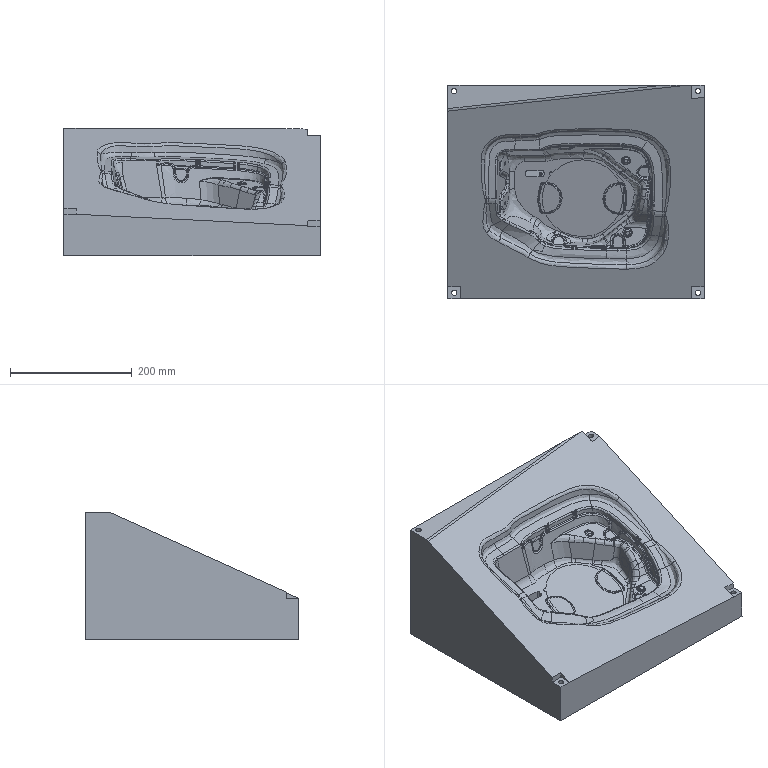NC program | NX | posted with a generic post | part box 420 x 350 x 208.3 mm
Lines 76212 to 77162 of 93858:
(CAVITY_MILL_COPY_COPY , TOOL : B10)
N152416 M6
N152418 G54
N152420 G17 G0 G90 X-24.596 Y68.606 S1900 M3
N152422 G43 Z220. H0
N152424 Z144.013
N152426 G94 G1 Z143.813 F3000.
N152428 X-24.626 Y69.131
N152430 G3 X-26.737 Y71.013 R2.
N152432 G1 X-27.419 Y70.974
N152434 G2 X-28.982 Y69.714 R8.488
N152436 G3 X-29.614 Y66.957 R2.
N152438 G1 X-29.446 Y66.689
N152440 Z144.013
N152442 G0 Z208.6
N152444 X-24.184 Y68.622
N152446 Z143.713
N152448 G1 Z143.513
N152450 X-24.214 Y69.156
N152452 G3 X-26.327 Y71.037 R2.
N152454 G1 X-27.167 Y70.988
N152456 G2 X-28.833 Y69.636 R8.726
N152458 G3 X-29.47 Y66.88 R2.
N152460 G1 X-29.3 Y66.608
N152462 Z143.713
N152464 G0 Z144.113
N152466 X-23.794 Y68.651
N152468 Z143.413
N152470 G1 Z143.213
N152472 X-23.818 Y69.15
N152474 G3 X-25.91 Y71.053 R2.
N152476 G1 X-26.569 Y71.022
N152478 X-26.917 Y71.002
N152480 G2 X-28.766 Y69.51 R8.706
N152482 G3 X-29.447 Y66.765 R2.
N152484 G1 X-29.282 Y66.491
N152486 Z143.413
N152488 G0 Z143.813
N152490 X-23.345 Y68.655
N152492 Z143.113
N152494 G1 Z142.913
N152496 X-23.365 Y69.155
N152498 G3 X-25.442 Y71.074 R2.
N152500 G1 X-26.179 Y71.045
N152502 X-26.699 Y71.014
N152504 G2 X-28.699 Y69.388 R8.526
N152506 G3 X-29.411 Y66.65 R2.
N152508 G1 X-29.25 Y66.377
N152510 Z143.113
N152512 G0 Z143.513
N152514 X-22.975 Y68.655
N152516 Z142.813
N152518 G1 Z142.613
N152520 X-23. Y69.154
N152522 G3 X-25.097 Y71.053 R2.
N152524 G1 X-26.52 Y70.982
N152526 G2 X-27.871 Y69.77 R8.475
N152528 G3 X-28.326 Y66.979 R2.
N152530 G1 X-28.141 Y66.722
N152532 Z142.813
N152534 G0 Z143.213
N152536 X-22.85 Y68.582
N152538 Z142.513
N152540 G1 Z142.313
N152542 X-22.875 Y69.084
N152544 G3 X-24.973 Y70.981 R2.
N152546 X-26.401 Y70.907 R693.689
N152548 G2 X-27.569 Y69.827 R8.285
N152550 G3 X-27.949 Y67.024 R2.
N152552 G1 X-27.76 Y66.775
N152554 Z142.513
N152556 G0 Z142.913
N152558 X-22.785 Y68.497
N152560 Z142.213
N152562 G1 Z142.013
N152564 X-22.809 Y68.998
N152566 G3 X-24.903 Y70.9 R2.
N152568 X-26.286 Y70.833 R1187.342
N152570 G2 X-27.347 Y69.835 R8.267
N152572 G3 X-27.683 Y67.027 R2.
N152574 G1 X-27.49 Y66.781
N152576 Z142.213
N152578 G0 Z142.613
N152580 X-22.687 Y68.421
N152582 Z141.913
N152584 G1 Z141.713
N152586 X-22.711 Y68.922
N152588 G3 X-24.804 Y70.824 R2.
N152590 X-26.172 Y70.758 R1216.244
N152592 G2 X-27.272 Y69.742 R8.44
N152594 G3 X-27.635 Y66.937 R2.
N152596 G1 X-27.442 Y66.687
N152598 Z141.913
N152600 G0 Z142.313
N152602 X-22.555 Y68.357
N152604 Z141.613
N152606 G1 Z141.413
N152608 X-22.581 Y68.862
N152610 G3 X-24.681 Y70.756 R2.
N152612 G1 X-26.066 Y70.684
N152614 G2 X-27.087 Y69.733 R8.336
N152616 G3 X-27.423 Y66.925 R2.
N152618 G1 X-27.23 Y66.678
N152620 Z141.613
N152622 G0 Z142.013
N152624 X-22.506 Y68.28
N152626 Z141.313
N152628 G1 Z141.113
N152630 X-22.531 Y68.779
N152632 G3 X-24.629 Y70.676 R2.
N152634 G1 X-25.967 Y70.609
N152636 G2 X-26.885 Y69.748 R8.451
N152638 G3 X-27.186 Y66.936 R2.
N152640 G1 X-26.987 Y66.69
N152642 Z141.313
N152644 G0 Z141.713
N152646 X-22.35 Y68.195
N152648 Z141.013
N152650 G1 Z140.813
N152652 X-22.373 Y68.696
N152654 G3 X-24.464 Y70.601 R2.
N152656 X-25.895 Y70.533 R1288.553
N152658 G2 X-26.753 Y69.72 R8.313
N152660 G3 X-27.03 Y66.905 R2.
N152662 G1 X-26.831 Y66.663
N152664 Z141.013
N152666 G0 Z141.413
N152668 X-22.395 Y68.125
N152670 Z140.713
N152672 G1 Z140.513
N152674 X-22.42 Y68.624
N152676 G3 X-24.518 Y70.522 R2.
N152678 G1 X-25.81 Y70.457
N152680 G2 X-26.608 Y69.701 R8.313
N152682 G3 X-26.871 Y66.885 R2.
N152684 G1 X-26.671 Y66.643
N152686 Z140.713
N152688 G0 Z141.113
N152690 X-22.336 Y68.049
N152692 Z140.413
N152694 G1 Z140.213
N152696 X-22.361 Y68.549
N152698 G3 X-24.459 Y70.445 R2.
N152700 G1 X-25.73 Y70.381
N152702 G2 X-26.499 Y69.657 R8.357
N152704 G3 X-26.763 Y66.841 R2.
N152706 G1 X-26.563 Y66.599
N152708 Z140.413
N152710 G0 Z140.813
N152712 X-22.29 Y67.968
N152714 Z140.113
N152716 G1 Z139.913
N152718 X-22.317 Y68.476
N152720 G3 X-24.418 Y70.369 R2.
N152722 G1 X-25.659 Y70.304
N152724 G2 X-26.372 Y69.632 R8.336
N152726 G3 X-26.621 Y66.815 R2.
N152728 G1 X-26.42 Y66.574
N152730 Z140.113
N152732 G0 Z140.513
N152734 X-22.224 Y67.897
N152736 Z139.813
N152738 G1 Z139.613
N152740 X-22.25 Y68.397
N152742 G3 X-24.35 Y70.291 R2.
N152744 G1 X-25.617 Y70.226
N152746 G2 X-26.283 Y69.593 R8.232
N152748 G3 X-26.515 Y66.774 R2.
N152750 G1 X-26.313 Y66.536
N152752 Z139.813
N152754 G0 Z140.213
N152756 X-22.246 Y67.818
N152758 Z139.513
N152760 G1 Z139.313
N152762 X-22.272 Y68.317
N152764 G3 X-24.373 Y70.21 R2.
N152766 G1 X-25.562 Y70.148
N152768 G2 X-26.205 Y69.543 R8.285
N152770 G3 X-26.441 Y66.725 R2.
N152772 G1 X-26.239 Y66.486
N152774 Z139.513
N152776 G0 Z139.913
N152778 X-22.277 Y67.737
N152780 Z139.213
N152782 G1 Z139.013
N152784 X-22.303 Y68.237
N152786 G3 X-24.406 Y70.129 R2.
N152788 G1 X-25.518 Y70.07
N152790 G2 X-26.098 Y69.523 R8.284
N152792 G3 X-26.318 Y66.704 R2.
N152794 G1 X-26.114 Y66.466
N152796 Z139.213
N152798 G0 Z139.613
N152800 X-22.359 Y67.654
N152802 Z138.913
N152804 G1 Z138.713
N152806 X-22.386 Y68.154
N152808 G3 X-24.489 Y70.044 R2.
N152810 G1 X-25.48 Y69.992
N152812 G2 X-26. Y69.5 R8.253
N152814 G3 X-26.202 Y66.679 R2.
N152816 G1 X-25.998 Y66.443
N152818 Z138.913
N152820 G0 Z139.313
N152822 X-22.463 Y67.559
N152824 Z138.614
N152826 G1 Z138.414
N152828 X-22.488 Y68.059
N152830 G3 X-24.585 Y69.957 R2.
N152832 G1 X-25.443 Y69.914
N152834 G2 X-25.905 Y69.478 R8.28
N152836 G3 X-26.096 Y66.656 R2.
N152838 G1 X-25.89 Y66.421
N152840 Z138.614
N152842 G0 Z139.013
N152844 X-21.214 Y67.536
N152846 Z138.314
N152848 G1 Z138.114
N152850 X-21.237 Y68.037
N152852 G3 X-23.329 Y69.941 R2.
N152854 X-25.423 Y69.84 R942.677
N152856 G2 X-26.653 Y68.814 R8.248
N152858 G3 X-27.182 Y66.035 R2.
N152860 G1 X-27.006 Y65.777
N152862 Z138.314
N152864 G0 Z138.714
N152866 X-21.185 Y67.466
N152868 Z138.014
N152870 G1 Z137.814
N152872 X-21.208 Y67.967
N152874 G3 X-23.298 Y69.873 R2.
N152876 X-25.387 Y69.774 R1000.498
N152878 G2 X-26.617 Y68.754 R8.221
N152880 G3 X-27.152 Y65.976 R2.
N152882 G1 X-26.977 Y65.718
N152884 Z138.014
N152886 G0 Z138.414
N152888 X-21.162 Y67.4
N152890 Z137.714
N152892 G1 Z137.514
N152894 X-21.185 Y67.901
N152896 G3 X-23.272 Y69.81 R2.
N152898 X-25.364 Y69.715 R1143.171
N152900 G2 X-26.596 Y68.694 R8.192
N152902 G3 X-27.133 Y65.917 R2.
N152904 G1 X-26.959 Y65.659
N152906 Z137.714
N152908 G0 Z138.114
N152910 X-21.658 Y67.322
N152912 Z137.414
N152914 G1 Z137.214
N152916 X-21.679 Y67.823
N152918 G3 X-23.762 Y69.736 R2.
N152920 G1 X-25.345 Y69.656
N152922 G2 X-26.217 Y68.892 R8.146
N152924 G3 X-26.604 Y66.09 R2.
N152926 G1 X-26.416 Y65.843
N152928 Z137.414
N152930 G0 Z137.814
N152932 X-21.11 Y67.287
N152934 Z137.114
N152936 G1 Z136.914
N152938 X-21.133 Y67.797
N152940 G3 X-23.221 Y69.704 R2.
N152942 X-25.326 Y69.596 R177.448
N152944 G2 X-26.544 Y68.585 R8.113
N152946 G3 X-27.079 Y65.807 R2.
N152948 G1 X-26.905 Y65.551
N152950 Z137.114
N152952 G0 Z137.514
N152954 X-21.097 Y67.234
N152956 Z136.814
N152958 G1 Z136.614
N152960 X-21.121 Y67.745
N152962 G3 X-23.213 Y69.648 R2.
N152964 X-25.307 Y69.537 R177.82
N152966 G2 X-26.521 Y68.531 R8.117
N152968 G3 X-27.057 Y65.754 R2.
N152970 G1 X-26.883 Y65.497
N152972 Z136.814
N152974 G0 Z137.214
N152976 X-21.105 Y67.182
N152978 Z136.514
N152980 G1 Z136.314
N152982 X-21.134 Y67.703
N152984 G3 X-23.24 Y69.59 R2.
N152986 G1 X-25.287 Y69.478
N152988 G2 X-26.497 Y68.479 R8.142
N152990 G3 X-27.035 Y65.703 R2.
N152992 G1 X-26.862 Y65.446
N152994 Z136.514
N152996 G0 Z136.914
N152998 X-21.072 Y67.128
N153000 Z136.214
N153002 G1 Z136.014
N153004 X-21.1 Y67.649
N153006 G3 X-23.207 Y69.537 R2.
N153008 G1 X-25.263 Y69.424
N153010 G2 X-26.306 Y68.535 R7.935
N153012 G3 X-26.773 Y65.745 R2.
N153014 G1 X-26.595 Y65.496
N153016 Z136.214
N153018 G0 Z136.614
N153020 X-21.053 Y67.073
N153022 Z135.914
N153024 G1 Z135.714
N153026 X-21.081 Y67.594
N153028 G3 X-23.186 Y69.483 R2.
N153030 G1 X-25.236 Y69.373
N153032 G2 X-26.275 Y68.492 R8.03
N153034 G3 X-26.745 Y65.703 R2.
N153036 G1 X-26.566 Y65.451
N153038 Z135.914
N153040 G0 Z136.314
N153042 X-21.023 Y67.019
N153044 Z135.614
N153046 G1 Z135.414
N153048 X-21.05 Y67.539
N153050 G3 X-23.154 Y69.43 R2.
N153052 G1 X-25.209 Y69.321
N153054 G2 X-26.186 Y68.483 R8.026
N153056 G3 X-26.628 Y65.689 R2.
N153058 G1 X-26.447 Y65.44
N153060 Z135.614
N153062 G0 Z136.014
N153064 X-20.996 Y66.965
N153066 Z135.314
N153068 G1 Z135.114
N153070 X-21.023 Y67.484
N153072 G3 X-23.124 Y69.377 R2.
N153074 G1 X-25.182 Y69.27
N153076 G2 X-26.172 Y68.423 R8.034
N153078 G3 X-26.619 Y65.63 R2.
N153080 G1 X-26.438 Y65.38
N153082 Z135.314
N153084 G0 Z135.714
N153086 X-20.969 Y66.911
N153088 Z135.014
N153090 G1 Z134.814
N153092 X-20.996 Y67.429
N153094 G3 X-23.096 Y69.324 R2.
N153096 G1 X-25.155 Y69.219
N153098 G2 X-26.164 Y68.358 R8.052
N153100 G3 X-26.62 Y65.567 R2.
N153102 G1 X-26.44 Y65.316
N153104 Z135.014
N153106 G0 Z135.414
N153108 X-20.944 Y66.856
N153110 Z134.714
N153112 G1 Z134.514
N153114 X-20.97 Y67.374
N153116 G3 X-23.069 Y69.271 R2.
N153118 G1 X-25.128 Y69.167
N153120 G2 X-26.167 Y68.287 R8.084
N153122 G3 X-26.637 Y65.498 R2.
N153124 G1 X-26.458 Y65.246
N153126 Z134.714
N153128 G0 Z135.114
N153130 X-20.919 Y66.802
N153132 Z134.414
N153134 G1 Z134.214
N153136 X-20.944 Y67.319
N153138 G3 X-23.041 Y69.218 R2.
N153140 G1 X-25.101 Y69.116
N153142 G2 X-26.17 Y68.216 R8.106
N153144 G3 X-26.653 Y65.429 R2.
N153146 G1 X-26.475 Y65.176
N153148 Z134.414
N153150 G0 Z134.814
N153152 X-20.87 Y66.741
N153154 Z134.114
N153156 G1 Z133.914
N153158 X-20.888 Y67.24
N153160 G3 X-22.96 Y69.166 R2.
N153162 G1 X-23.054 Y69.163
N153164 X-25.075 Y69.064
N153166 G2 X-26.159 Y68.154 R8.108
N153168 G3 X-26.65 Y65.368 R2.
N153170 G1 X-26.472 Y65.114
N153172 Z134.114
N153174 G0 Z134.514
N153176 X-20.828 Y66.69
N153178 Z133.814
N153180 G1 Z133.614
N153182 X-20.846 Y67.189
N153184 G3 X-22.918 Y69.115 R2.
N153186 G1 X-23.054 Y69.11
N153188 X-25.049 Y69.013
N153190 G2 X-26.12 Y68.111 R8.099
N153192 G3 X-26.605 Y65.325 R2.
N153194 G1 X-26.427 Y65.071
N153196 Z133.814
N153198 G0 Z134.214
N153200 X-20.796 Y66.638
N153202 Z133.515
N153204 G1 Z133.315
N153206 X-20.814 Y67.138
N153208 G3 X-22.885 Y69.063 R2.
N153210 G1 X-23.054 Y69.057
N153212 X-25.023 Y68.961
N153214 G2 X-26.095 Y68.06 R8.111
N153216 G3 X-26.581 Y65.273 R2.
N153218 G1 X-26.403 Y65.02
N153220 Z133.515
N153222 G0 Z133.914
N153224 X-20.772 Y66.586
N153226 Z133.215
N153228 G1 Z133.015
N153230 X-20.791 Y67.086
N153232 G3 X-22.862 Y69.011 R2.
N153234 G1 X-23.054 Y69.004
N153236 X-24.997 Y68.91
N153238 G2 X-26.073 Y68.007 R8.129
N153240 G3 X-26.561 Y65.221 R2.
N153242 G1 X-26.383 Y64.967
N153244 Z133.215
N153246 G0 Z133.615
N153248 X-20.746 Y66.534
N153250 Z132.915
N153252 G1 Z132.715
N153254 X-20.764 Y67.034
N153256 G3 X-22.836 Y68.959 R2.
N153258 G1 X-23.054 Y68.952
N153260 X-24.971 Y68.859
N153262 G2 X-26.031 Y67.966 R8.119
N153264 G3 X-26.512 Y65.179 R2.
N153266 G1 X-26.333 Y64.926
N153268 Z132.915
N153270 G0 Z133.315
N153272 X-20.722 Y66.482
N153274 Z132.615
N153276 G1 Z132.415
N153278 X-20.74 Y66.982
N153280 G3 X-22.812 Y68.907 R2.
N153282 G1 X-23.054 Y68.899
N153284 X-24.945 Y68.807
N153286 G2 X-25.995 Y67.922 R8.129
N153288 G3 X-26.474 Y65.134 R2.
N153290 G1 X-26.295 Y64.881
N153292 Z132.615
N153294 G0 Z133.015
N153296 X-20.697 Y66.43
N153298 Z132.315
N153300 G1 Z132.115
N153302 X-20.715 Y66.93
N153304 G3 X-22.787 Y68.856 R2.
N153306 G1 X-23.054 Y68.846
N153308 X-24.919 Y68.756
N153310 G2 X-25.962 Y67.876 R8.13
N153312 G3 X-26.438 Y65.088 R2.
N153314 G1 X-26.258 Y64.834
N153316 Z132.315
N153318 G0 Z132.715
N153320 X-20.672 Y66.378
N153322 Z132.015
N153324 G1 Z131.815
N153326 X-20.691 Y66.878
N153328 G3 X-22.762 Y68.804 R2.
N153330 G1 X-23.054 Y68.793
N153332 X-24.893 Y68.704
N153334 G2 X-25.927 Y67.831 R8.138
N153336 G3 X-26.399 Y65.042 R2.
N153338 G1 X-26.219 Y64.789
N153340 Z132.015
N153342 G0 Z132.415
N153344 X-20.724 Y66.323
N153346 Z131.715
N153348 G1 Z131.515
N153350 X-20.742 Y66.823
N153352 G3 X-22.814 Y68.749 R2.
N153354 G1 X-23.054 Y68.74
N153356 X-24.867 Y68.653
N153358 G2 X-25.893 Y67.786 R8.143
N153360 G3 X-26.362 Y64.996 R2.
N153362 G1 X-26.182 Y64.744
N153364 Z131.715
N153366 G0 Z132.115
N153368 X-20.771 Y66.269
N153370 Z131.415
N153372 G1 Z131.215
N153374 X-20.789 Y66.768
N153376 G3 X-22.861 Y68.694 R2.
N153378 G1 X-23.054 Y68.687
N153380 X-24.84 Y68.601
N153382 G2 X-25.863 Y67.738 R8.162
N153384 G3 X-26.332 Y64.949 R2.
N153386 G1 X-26.152 Y64.695
N153388 Z131.415
N153390 G0 Z131.815
N153392 X-20.796 Y66.215
N153394 Z131.115
N153396 G1 Z130.915
N153398 X-20.815 Y66.715
N153400 G3 X-22.886 Y68.64 R2.
N153402 G1 X-23.054 Y68.634
N153404 X-24.814 Y68.55
N153406 G2 X-25.827 Y67.694 R8.173
N153408 G3 X-26.292 Y64.904 R2.
N153410 G1 X-26.112 Y64.651
N153412 Z131.115
N153414 G0 Z131.515
N153416 X-20.824 Y66.161
N153418 Z130.815
N153420 G1 Z130.615
N153422 X-20.842 Y66.661
N153424 G3 X-22.914 Y68.587 R2.
N153426 G1 X-23.054 Y68.581
N153428 X-24.788 Y68.499
N153430 G2 X-25.876 Y67.591 R8.183
N153432 G3 X-26.372 Y64.806 R2.
N153434 G1 X-26.194 Y64.551
N153436 Z130.815
N153438 G0 Z131.215
N153440 X-20.828 Y66.108
N153442 Z130.515
N153444 G1 Z130.315
N153446 X-20.846 Y66.608
N153448 G3 X-22.917 Y68.534 R2.
N153450 G1 X-23.054 Y68.529
N153452 X-24.762 Y68.447
N153454 G2 X-25.754 Y67.608 R8.2
N153456 G3 X-26.211 Y64.817 R2.
N153458 G1 X-26.029 Y64.564
N153460 Z130.515
N153462 G0 Z130.915
N153464 X-20.838 Y66.055
N153466 Z130.215
N153468 G1 Z130.015
N153470 X-20.857 Y66.554
N153472 G3 X-22.928 Y68.48 R2.
N153474 G1 X-23.054 Y68.476
N153476 X-24.736 Y68.396
N153478 G2 X-25.713 Y67.568 R8.212
N153480 G3 X-26.164 Y64.776 R2.
N153482 G1 X-25.982 Y64.523
N153484 Z130.215
N153486 G0 Z130.615
N153488 X-20.847 Y66.002
N153490 Z129.915
N153492 G1 Z129.715
N153494 X-20.865 Y66.501
N153496 G3 X-22.937 Y68.427 R2.
N153498 G1 X-23.054 Y68.423
N153500 X-24.71 Y68.344
N153502 G2 X-25.656 Y67.537 R8.164
N153504 G3 X-26.095 Y64.743 R2.
N153506 G1 X-25.912 Y64.492
N153508 Z129.915
N153510 G0 Z130.315
N153512 X-20.855 Y65.948
N153514 Z129.615
N153516 G1 Z129.415
N153518 X-20.873 Y66.448
N153520 G3 X-22.945 Y68.374 R2.
N153522 G1 X-23.054 Y68.37
N153524 X-24.684 Y68.293
N153526 G2 X-25.63 Y67.488 R8.232
N153528 G3 X-26.07 Y64.694 R2.
N153530 G1 X-25.887 Y64.442
N153532 Z129.615
N153534 G0 Z130.015
N153536 X-20.861 Y65.895
N153538 Z129.315
N153540 G1 Z129.115
N153542 X-20.879 Y66.395
N153544 G3 X-22.951 Y68.321 R2.
N153546 G1 X-23.054 Y68.317
N153548 X-24.658 Y68.241
N153550 G2 X-25.589 Y67.448 R8.242
N153552 G3 X-26.023 Y64.653 R2.
N153554 G1 X-25.839 Y64.401
N153556 Z129.315
N153558 G0 Z129.715
N153560 X-20.867 Y65.842
N153562 Z129.015
N153564 G1 Z128.815
N153566 X-20.885 Y66.342
N153568 G3 X-22.957 Y68.268 R2.
N153570 G1 X-23.054 Y68.264
N153572 X-24.632 Y68.19
N153574 G2 X-25.555 Y67.404 R8.253
N153576 G3 X-25.988 Y64.609 R2.
N153578 G1 X-25.803 Y64.357
N153580 Z129.015
N153582 G0 Z129.415
N153584 X-21.65 Y65.755
N153586 Z128.715
N153588 G1 Z128.515
N153590 X-21.669 Y66.254
N153592 G3 X-23.742 Y68.179 R2.
N153594 G1 X-23.835 Y68.175
N153596 X-24.606 Y68.138
N153598 G2 X-25.07 Y67.711 R8.17
N153600 G3 X-25.297 Y64.891 R2.
N153602 G1 X-25.095 Y64.655
N153604 Z128.715
N153606 G0 Z129.115
N153608 X-21.625 Y65.703
N153610 Z128.416
N153612 G1 Z128.216
N153614 X-21.644 Y66.202
N153616 G3 X-23.717 Y68.127 R2.
N153618 G1 X-23.835 Y68.123
N153620 X-24.58 Y68.087
N153622 G2 X-25.045 Y67.659 R8.17
N153624 G3 X-25.271 Y64.84 R2.
N153626 G1 X-25.07 Y64.603
N153628 Z128.416
N153630 G0 Z128.815
N153632 X-21.6 Y65.651
N153634 Z128.116
N153636 G1 Z127.916
N153638 X-21.619 Y66.151
N153640 G3 X-23.692 Y68.075 R2.
N153642 G1 X-23.835 Y68.07
N153644 X-24.554 Y68.035
N153646 G2 X-25.018 Y67.608 R8.168
N153648 G3 X-25.244 Y64.789 R2.
N153650 G1 X-25.043 Y64.552
N153652 Z128.116
N153654 G0 Z128.516
N153656 X-21.575 Y65.599
N153658 Z127.816
N153660 G1 Z127.616
N153662 X-21.594 Y66.099
N153664 G3 X-23.667 Y68.023 R2.
N153666 G1 X-23.835 Y68.017
N153668 X-24.528 Y67.984
N153670 G2 X-24.992 Y67.557 R8.173
N153672 G3 X-25.219 Y64.737 R2.
N153674 G1 X-25.018 Y64.5
N153676 Z127.816
N153678 G0 Z128.216
N153680 X-21.55 Y65.547
N153682 Z127.516
N153684 G1 Z127.316
N153686 X-21.569 Y66.047
N153688 G3 X-23.641 Y67.971 R2.
N153690 G1 X-23.835 Y67.964
N153692 X-24.502 Y67.932
N153694 G2 X-24.964 Y67.506 R8.149
N153696 G3 X-25.187 Y64.687 R2.
N153698 G1 X-24.986 Y64.451
N153700 Z127.516
N153702 G0 Z127.916
N153704 X-21.513 Y65.496
N153706 Z127.216
N153708 G1 Z127.016
N153710 X-21.531 Y65.995
N153712 G3 X-23.604 Y67.92 R2.
N153714 G1 X-23.835 Y67.911
N153716 X-24.476 Y67.881
N153718 G2 X-24.95 Y67.443 R8.125
N153720 G3 X-25.177 Y64.624 R2.
N153722 G1 X-24.976 Y64.388
N153724 Z127.216
N153726 G0 Z127.616
N153728 X-21.5 Y65.443
N153730 Z126.916
N153732 G1 Z126.716
N153734 X-21.519 Y65.943
N153736 G3 X-23.592 Y67.868 R2.
N153738 G1 X-23.835 Y67.858
N153740 X-24.448 Y67.829
N153742 G2 X-24.932 Y67.38 R7.975
N153744 G3 X-25.158 Y64.561 R2.
N153746 G1 X-24.959 Y64.327
N153748 Z126.916
N153750 G0 Z127.316
N153752 X-21.449 Y65.392
N153754 Z126.616
N153756 G1 Z126.416
N153758 X-21.467 Y65.892
N153760 G3 X-23.54 Y67.817 R2.
N153762 G1 X-23.835 Y67.806
N153764 X-24.421 Y67.778
N153766 G2 X-24.937 Y67.3 R7.939
N153768 G3 X-25.173 Y64.482 R2.
N153770 G1 X-24.975 Y64.248
N153772 Z126.616
N153774 G0 Z127.016
N153776 X-21.328 Y65.344
N153778 Z126.316
N153780 G1 Z126.116
N153782 X-21.346 Y65.844
N153784 G3 X-23.419 Y67.768 R2.
N153786 G1 X-23.835 Y67.753
N153788 X-24.373 Y67.727
N153790 G2 X-24.999 Y67.163 R8.033
N153792 G3 X-25.293 Y64.35 R2.
N153794 G1 X-25.099 Y64.111
N153796 Z126.316
N153798 G0 Z126.716
N153800 X-21.468 Y65.291
N153802 Z126.016
N153804 G1 Z125.816
N153806 X-21.492 Y65.804
N153808 G3 X-23.581 Y67.711 R2.
N153810 G1 X-24.326 Y67.677
N153812 G2 X-24.803 Y67.237 R8.039
N153814 G3 X-25.03 Y64.417 R2.
N153816 G1 X-24.83 Y64.182
N153818 Z126.016
N153820 G0 Z126.416
N153822 X-21.414 Y65.235
N153824 Z125.716
N153826 G1 Z125.516
N153828 X-21.433 Y65.735
N153830 G3 X-23.505 Y67.659 R2.
N153832 G1 X-23.835 Y67.647
N153834 X-24.278 Y67.626
N153836 G2 X-24.799 Y67.147 R7.995
N153838 G3 X-25.043 Y64.329 R2.
N153840 G1 X-24.845 Y64.094
N153842 Z125.716
N153844 G0 Z126.116
N153846 X-21.32 Y65.186
N153848 Z125.416
N153850 G1 Z125.216
N153852 X-21.338 Y65.686
N153854 G3 X-23.411 Y67.61 R2.
N153856 G1 X-23.835 Y67.594
N153858 X-24.209 Y67.577
N153860 G2 X-24.78 Y67.058 R8.04
N153862 G3 X-25.05 Y64.243 R2.
N153864 G1 X-24.854 Y64.005
N153866 Z125.416
N153868 G0 Z125.816
N153870 X-21.216 Y65.135
N153872 Z125.116
N153874 G1 Z124.916
N153876 X-21.235 Y65.635
N153878 G3 X-23.308 Y67.559 R2.
N153880 G1 X-24.101 Y67.529
N153882 G2 X-24.725 Y66.979 R8.316
N153884 G3 X-25.044 Y64.168 R2.
N153886 G1 X-24.848 Y63.923
N153888 Z125.116
N153890 G0 Z125.516
N153892 X-21.067 Y65.098
N153894 Z124.816
N153896 G1 Z124.616
N153898 X-21.088 Y65.605
N153900 G3 X-23.173 Y67.517 R2.
N153902 G1 X-23.996 Y67.481
N153904 G2 X-24.677 Y66.894 R8.526
N153906 G3 X-25.037 Y64.089 R2.
N153908 G1 X-24.843 Y63.838
N153910 Z124.816
N153912 G0 Z125.216
N153914 X-20.941 Y65.05
N153916 Z124.516
N153918 G1 Z124.316
N153920 X-20.963 Y65.558
N153922 G3 X-23.048 Y67.469 R2.
N153924 G1 X-23.892 Y67.433
N153926 G2 X-24.641 Y66.798 R8.595
N153928 G3 X-25.035 Y63.997 R2.
N153930 G1 X-24.843 Y63.743
N153932 Z124.516
N153934 G0 Z124.916
N153936 X-20.801 Y65.002
N153938 Z124.216
N153940 G1 Z124.016
N153942 X-20.823 Y65.51
N153944 G3 X-22.907 Y67.423 R2.
N153946 G1 X-23.775 Y67.385
N153948 G2 X-24.63 Y66.675 R8.668
N153950 G3 X-25.072 Y63.882 R2.
N153952 G1 X-24.884 Y63.623
N153954 Z124.216
N153956 G0 Z124.616
N153958 X-20.645 Y64.955
N153960 Z123.916
N153962 G1 Z123.716
N153964 X-20.667 Y65.464
N153966 G3 X-22.751 Y67.377 R2.
N153968 G1 X-23.619 Y67.339
N153970 G2 X-24.633 Y66.532 R8.953
N153972 G3 X-25.154 Y63.752 R2.
N153974 G1 X-24.971 Y63.485
N153976 Z123.916
N153978 G0 Z124.316
N153980 X-20.473 Y64.908
N153982 Z123.616
N153984 G1 Z123.416
N153986 X-20.495 Y65.418
N153988 G3 X-22.578 Y67.331 R2.
N153990 G1 X-23.463 Y67.293
N153992 G2 X-24.611 Y66.399 R8.841
N153994 G3 X-25.189 Y63.63 R2.
N153996 G1 X-25.013 Y63.36
N153998 Z123.616
N154000 G0 Z124.016
N154002 X-20.302 Y64.861
N154004 Z123.317
N154006 G1 Z123.117
N154008 X-20.324 Y65.372
N154010 G3 X-22.406 Y67.286 R2.
N154012 G1 X-23.265 Y67.249
N154014 G2 X-24.57 Y66.276 R9.205
N154016 G3 X-25.223 Y63.524 R2.
N154018 G1 X-25.051 Y63.244
N154020 Z123.317
N154022 G0 Z123.716
N154024 X-20.113 Y64.816
N154026 Z123.017
N154028 G1 Z122.817
N154030 X-20.131 Y65.315
N154032 G3 X-22.203 Y67.241 R2.
N154034 G1 X-23.057 Y67.206
N154036 G2 X-24.616 Y66.1 R9.526
N154038 G3 X-25.369 Y63.374 R2.
N154040 G1 X-25.205 Y63.085
N154042 Z123.017
N154044 G0 Z123.417
N154046 X-19.908 Y64.77
N154048 Z122.717
N154050 G1 Z122.517
N154052 X-19.926 Y65.27
N154054 G3 X-21.998 Y67.195 R2.
N154056 G1 X-22.272 Y67.185
N154058 X-22.792 Y67.164
N154060 G2 X-24.99 Y65.779 R10.597
N154062 G3 X-25.949 Y63.119 R2.
N154064 G1 X-25.802 Y62.805
N154066 Z122.717
N154068 G0 Z123.117
N154070 X-19.683 Y64.725
N154072 Z122.417
N154074 G1 Z122.217
N154076 X-19.701 Y65.225
N154078 G3 X-21.774 Y67.15 R2.
N154080 G1 X-22.518 Y67.122
N154082 G2 X-24.976 Y65.657 R12.08
N154084 G3 X-25.989 Y63.016 R2.
N154086 G1 X-25.847 Y62.697
N154088 Z122.417
N154090 G0 Z122.817
N154092 X-19.428 Y64.682
N154094 Z122.117
N154096 G1 Z121.917
N154098 X-19.447 Y65.182
N154100 G3 X-21.519 Y67.107 R2.
N154102 G1 X-22.245 Y67.08
N154104 G2 X-24.842 Y65.582 R11.939
N154106 G3 X-25.912 Y62.963 R2.
N154108 G1 X-25.773 Y62.631
N154110 Z122.117
N154112 G0 Z123.217
N154114 X77.643 Y53.74
N154116 Z121.217
N154118 G1 Z121.017
N154120 G3 X80.036 Y54.931 R2.
N154122 G2 X80.346 Y55.264 R0.627
N154124 X82.481 Y55.241 R1.437
N154126 G3 X85.123 Y54.92 R2.
N154128 G1 Z121.217
N154130 G0 Z121.617
N154132 X99.419 Y59.382
N154134 Z121.217
N154136 G1 Z121.017
N154138 X99.625 Y59.92
N154140 G3 X98.474 Y62.504 R2.
N154142 G1 X98.44 Y62.517
N154144 X58.723 Y56.193
N154146 G2 X55.461 Y56.234 R21.912
N154148 G3 X53.294 Y54.416 R2.
N154150 G1 X53.258 Y53.999
N154152 Z121.217
N154154 G0 Z121.617
N154156 X76.778 Y50.866
N154158 Z120.917
N154160 G1 Z120.717
N154162 G3 X77.996 Y53.408 R2.
N154164 G2 X77.905 Y53.91 R1.641
N154166 X78.508 Y55.812 R2.792
N154168 X84.554 Y55.829 R3.867
N154170 X84.581 Y53.531 R1.814
N154172 G3 X84.901 Y50.715 R2.
N154174 G1 Z120.917
N154176 G0 Z121.317
N154178 X100.805 Y58.63
N154180 Z120.917
N154182 G1 Z120.717
N154184 X101.042 Y59.177
N154186 G3 X100.002 Y61.807 R2.
N154188 G1 X99.953 Y61.828
N154190 X59.518 Y55.391
N154192 G2 X56.482 Y55.433 R18.77
N154194 G3 X54.301 Y53.631 R2.
N154196 G1 X54.263 Y53.227
N154198 Z120.917
N154200 G0 Z121.317
N154202 X76.151 Y49.646
N154204 Z120.617
N154206 G1 Z120.417
N154208 X76.217 Y49.68
N154210 G3 X77.046 Y52.384 R2.
N154212 G2 X76.766 Y53.489 R2.41
N154214 X79.402 Y57.627 R4.494
N154216 G1 X60.265 Y54.58
N154218 G2 X57.293 Y54.641 R16.305
N154220 G3 X55.082 Y52.877 R2.
N154222 G1 X55.038 Y52.486
N154224 Z120.617
N154226 G0 Z121.017
N154228 X75.651 Y48.665
N154230 Z120.317
N154232 G1 Z120.117
N154234 X75.741 Y48.719
N154236 G3 X76.431 Y51.461 R2.
N154238 G2 X76.165 Y52.059 R2.763
N154240 X76.848 Y56.291 R4.79
N154242 G1 X60.995 Y53.767
N154244 G2 X58.103 Y53.846 R13.352
N154246 G3 X55.85 Y52.135 R2.
N154248 G1 X55.799 Y51.759
N154250 Z120.317
N154252 G0 Z120.717
N154254 X77.992 Y46.7
N154256 Z120.017
N154258 G1 Z119.817
N154260 X78.051 Y46.812
N154262 G3 X77.218 Y49.514 R2.
N154264 G2 X76.165 Y50.436 R3.039
N154266 X75.593 Y55.162 R5.084
N154268 G1 X61.712 Y52.952
N154270 G2 X58.77 Y53.062 R14.266
N154272 G3 X56.509 Y51.363 R2.
N154274 G1 X56.456 Y50.986
N154276 Z120.017
N154278 G0 Z120.417
N154280 X75.035 Y47.02
N154282 Z119.717
N154284 G1 Z119.517
N154286 X75.218 Y47.149
N154288 G3 X75.701 Y49.936 R2.
N154290 G2 X74.778 Y54.103 R5.535
N154292 G1 X62.423 Y52.136
N154294 G2 X59.634 Y52.225 R11.453
N154296 G3 X57.351 Y50.555 R2.
N154298 G1 X57.296 Y50.201
N154300 Z119.717
N154302 G0 Z120.117
N154304 X74.456 Y46.641
N154306 Z119.417
N154308 G1 Z119.217
N154310 X74.681 Y46.791